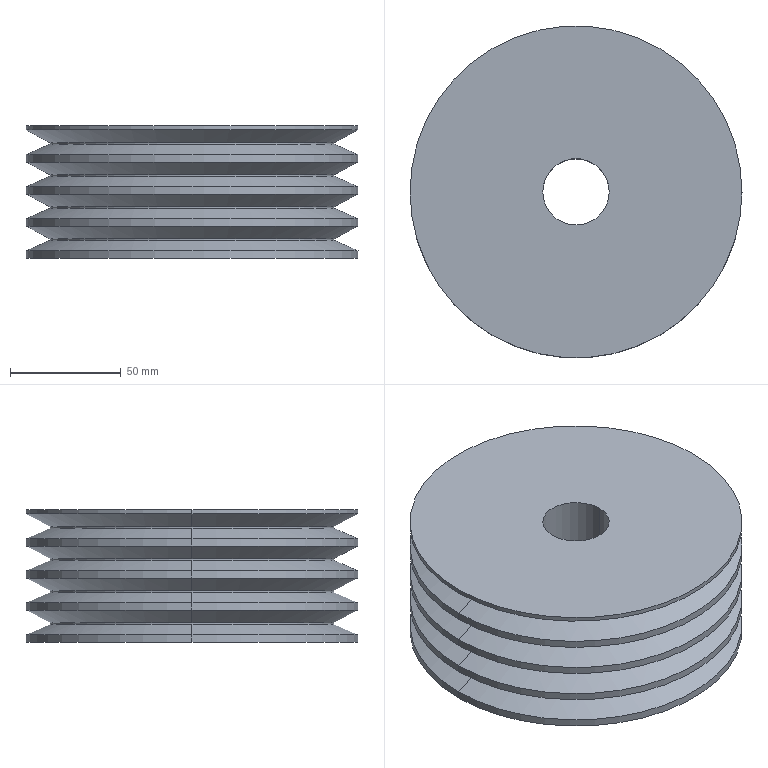Part | SolidWorks | features Extrusion 1, RevCut 1 | 1 solid | 38 faces | box 150 x 150 x 60 mm | volume 903652 mm3 | cylinder 20 | cone 16 | plane 2 | commonest cylinder face diameters 150 x10 128.527 x8 30 x2
STEP:
#1=CARTESIAN_POINT('',(75.,0.,17.907));
#2=VERTEX_POINT('',#1);
#3=CARTESIAN_POINT('',(-75.,0.,17.907));
#4=VERTEX_POINT('',#3);
#5=CARTESIAN_POINT('',(0.,0.,17.907));
#6=DIRECTION('',(0.,0.,1.));
#7=DIRECTION('',(1.,0.,0.));
#8=AXIS2_PLACEMENT_3D('',#5,#6,#7);
#9=CIRCLE('',#8,75.);
#10=EDGE_CURVE('',#2,#4,#9,.T.);
#11=ORIENTED_EDGE('',*,*,#10,.F.);
#12=CARTESIAN_POINT('',(75.,0.,14.583));
#13=VERTEX_POINT('',#12);
#14=CARTESIAN_POINT('',(75.,0.,60.));
#15=DIRECTION('',(0.,0.,-1.));
#16=VECTOR('',#15,1000.);
#17=LINE('',#14,#16);
#18=EDGE_CURVE('',#2,#13,#17,.T.);
#19=ORIENTED_EDGE('',*,*,#18,.T.);
#20=CARTESIAN_POINT('',(-75.,0.,14.583));
#21=VERTEX_POINT('',#20);
#22=CARTESIAN_POINT('',(0.,0.,14.583));
#23=DIRECTION('',(0.,0.,1.));
#24=DIRECTION('',(1.,0.,0.));
#25=AXIS2_PLACEMENT_3D('',#22,#23,#24);
#26=CIRCLE('',#25,75.);
#27=EDGE_CURVE('',#13,#21,#26,.T.);
#28=ORIENTED_EDGE('',*,*,#27,.T.);
#29=CARTESIAN_POINT('',(-75.,0.,60.));
#30=DIRECTION('',(0.,0.,-1.));
#31=VECTOR('',#30,1000.);
#32=LINE('',#29,#31);
#33=EDGE_CURVE('',#4,#21,#32,.T.);
#34=ORIENTED_EDGE('',*,*,#33,.F.);
#35=EDGE_LOOP('',(#11,#19,#28,#34));
#36=FACE_OUTER_BOUND('',#35,.T.);
#37=CARTESIAN_POINT('',(0.,0.,60.));
#38=DIRECTION('',(0.,0.,-1.));
#39=DIRECTION('',(-1.,0.,0.));
#40=AXIS2_PLACEMENT_3D('',#37,#38,#39);
#41=CYLINDRICAL_SURFACE('',#40,75.);
#42=ADVANCED_FACE('',(#36),#41,.T.);
#43=CARTESIAN_POINT('',(64.263,0.,22.613));
#44=VERTEX_POINT('',#43);
#45=CARTESIAN_POINT('',(-64.263,0.,22.613));
#46=VERTEX_POINT('',#45);
#47=CARTESIAN_POINT('',(0.,0.,22.613));
#48=DIRECTION('',(0.,0.,1.));
#49=DIRECTION('',(1.,0.,0.));
#50=AXIS2_PLACEMENT_3D('',#47,#48,#49);
#51=CIRCLE('',#50,64.263);
#52=EDGE_CURVE('',#44,#46,#51,.T.);
#53=ORIENTED_EDGE('',*,*,#52,.T.);
#54=CARTESIAN_POINT('',(-64.263,0.,23.348));
#55=VERTEX_POINT('',#54);
#56=CARTESIAN_POINT('',(-64.263,0.,0.));
#57=DIRECTION('',(0.,0.,1.));
#58=VECTOR('',#57,1000.);
#59=LINE('',#56,#58);
#60=EDGE_CURVE('',#46,#55,#59,.T.);
#61=ORIENTED_EDGE('',*,*,#60,.T.);
#62=CARTESIAN_POINT('',(64.263,0.,23.348));
#63=VERTEX_POINT('',#62);
#64=CARTESIAN_POINT('',(0.,0.,23.348));
#65=DIRECTION('',(0.,0.,1.));
#66=DIRECTION('',(1.,0.,0.));
#67=AXIS2_PLACEMENT_3D('',#64,#65,#66);
#68=CIRCLE('',#67,64.263);
#69=EDGE_CURVE('',#63,#55,#68,.T.);
#70=ORIENTED_EDGE('',*,*,#69,.F.);
#71=CARTESIAN_POINT('',(64.263,0.,0.));
#72=DIRECTION('',(0.,0.,1.));
#73=VECTOR('',#72,1000.);
#74=LINE('',#71,#73);
#75=EDGE_CURVE('',#44,#63,#74,.T.);
#76=ORIENTED_EDGE('',*,*,#75,.F.);
#77=EDGE_LOOP('',(#53,#61,#70,#76));
#78=FACE_OUTER_BOUND('',#77,.T.);
#79=CARTESIAN_POINT('',(0.,0.,0.));
#80=DIRECTION('',(0.,0.,1.));
#81=DIRECTION('',(1.,0.,0.));
#82=AXIS2_PLACEMENT_3D('',#79,#80,#81);
#83=CYLINDRICAL_SURFACE('',#82,64.263);
#84=ADVANCED_FACE('',(#78),#83,.T.);
#85=ORIENTED_EDGE('',*,*,#69,.T.);
#86=CARTESIAN_POINT('',(-75.,0.,29.063));
#87=VERTEX_POINT('',#86);
#88=CARTESIAN_POINT('',(-75.,0.,29.063));
#89=DIRECTION('',(-0.8827,0.,0.4699));
#90=VECTOR('',#89,1000.);
#91=LINE('',#88,#90);
#92=EDGE_CURVE('',#55,#87,#91,.T.);
#93=ORIENTED_EDGE('',*,*,#92,.T.);
#94=CARTESIAN_POINT('',(75.,0.,29.063));
#95=VERTEX_POINT('',#94);
#96=CARTESIAN_POINT('',(0.,0.,29.063));
#97=DIRECTION('',(0.,0.,1.));
#98=DIRECTION('',(1.,0.,0.));
#99=AXIS2_PLACEMENT_3D('',#96,#97,#98);
#100=CIRCLE('',#99,75.);
#101=EDGE_CURVE('',#95,#87,#100,.T.);
#102=ORIENTED_EDGE('',*,*,#101,.F.);
#103=CARTESIAN_POINT('',(75.,0.,29.063));
#104=DIRECTION('',(0.8827,0.,0.4699));
#105=VECTOR('',#104,1000.);
#106=LINE('',#103,#105);
#107=EDGE_CURVE('',#63,#95,#106,.T.);
#108=ORIENTED_EDGE('',*,*,#107,.F.);
#109=EDGE_LOOP('',(#85,#93,#102,#108));
#110=FACE_OUTER_BOUND('',#109,.T.);
#111=CARTESIAN_POINT('',(0.,0.,29.063));
#112=DIRECTION('',(0.,0.,1.));
#113=DIRECTION('',(1.,0.,0.));
#114=AXIS2_PLACEMENT_3D('',#111,#112,#113);
#115=CONICAL_SURFACE('',#114,75.,1.082);
#116=ADVANCED_FACE('',(#110),#115,.T.);
#117=ORIENTED_EDGE('',*,*,#52,.F.);
#118=CARTESIAN_POINT('',(64.263,0.,22.613));
#119=DIRECTION('',(0.9159,0.,-0.4015));
#120=VECTOR('',#119,1000.);
#121=LINE('',#118,#120);
#122=EDGE_CURVE('',#44,#2,#121,.T.);
#123=ORIENTED_EDGE('',*,*,#122,.T.);
#124=ORIENTED_EDGE('',*,*,#10,.T.);
#125=CARTESIAN_POINT('',(-64.263,0.,22.613));
#126=DIRECTION('',(-0.9159,0.,-0.4015));
#127=VECTOR('',#126,1000.);
#128=LINE('',#125,#127);
#129=EDGE_CURVE('',#46,#4,#128,.T.);
#130=ORIENTED_EDGE('',*,*,#129,.F.);
#131=EDGE_LOOP('',(#117,#123,#124,#130));
#132=FACE_OUTER_BOUND('',#131,.T.);
#133=CARTESIAN_POINT('',(0.,0.,22.613));
#134=DIRECTION('',(0.,0.,-1.));
#135=DIRECTION('',(-1.,0.,0.));
#136=AXIS2_PLACEMENT_3D('',#133,#134,#135);
#137=CONICAL_SURFACE('',#136,64.263,1.158);
#138=ADVANCED_FACE('',(#132),#137,.T.);
#139=CARTESIAN_POINT('',(75.,0.,32.387));
#140=VERTEX_POINT('',#139);
#141=CARTESIAN_POINT('',(-75.,0.,32.387));
#142=VERTEX_POINT('',#141);
#143=CARTESIAN_POINT('',(0.,0.,32.387));
#144=DIRECTION('',(0.,0.,1.));
#145=DIRECTION('',(1.,0.,0.));
#146=AXIS2_PLACEMENT_3D('',#143,#144,#145);
#147=CIRCLE('',#146,75.);
#148=EDGE_CURVE('',#140,#142,#147,.T.);
#149=ORIENTED_EDGE('',*,*,#148,.F.);
#150=CARTESIAN_POINT('',(75.,0.,60.));
#151=DIRECTION('',(0.,0.,-1.));
#152=VECTOR('',#151,1000.);
#153=LINE('',#150,#152);
#154=EDGE_CURVE('',#140,#95,#153,.T.);
#155=ORIENTED_EDGE('',*,*,#154,.T.);
#156=ORIENTED_EDGE('',*,*,#101,.T.);
#157=CARTESIAN_POINT('',(-75.,0.,60.));
#158=DIRECTION('',(0.,0.,-1.));
#159=VECTOR('',#158,1000.);
#160=LINE('',#157,#159);
#161=EDGE_CURVE('',#142,#87,#160,.T.);
#162=ORIENTED_EDGE('',*,*,#161,.F.);
#163=EDGE_LOOP('',(#149,#155,#156,#162));
#164=FACE_OUTER_BOUND('',#163,.T.);
#165=CARTESIAN_POINT('',(0.,0.,60.));
#166=DIRECTION('',(0.,0.,-1.));
#167=DIRECTION('',(-1.,0.,0.));
#168=AXIS2_PLACEMENT_3D('',#165,#166,#167);
#169=CYLINDRICAL_SURFACE('',#168,75.);
#170=ADVANCED_FACE('',(#164),#169,.T.);
#171=CARTESIAN_POINT('',(64.263,0.,37.093));
#172=VERTEX_POINT('',#171);
#173=CARTESIAN_POINT('',(-64.263,0.,37.093));
#174=VERTEX_POINT('',#173);
#175=CARTESIAN_POINT('',(0.,0.,37.093));
#176=DIRECTION('',(0.,0.,1.));
#177=DIRECTION('',(1.,0.,0.));
#178=AXIS2_PLACEMENT_3D('',#175,#176,#177);
#179=CIRCLE('',#178,64.263);
#180=EDGE_CURVE('',#172,#174,#179,.T.);
#181=ORIENTED_EDGE('',*,*,#180,.T.);
#182=CARTESIAN_POINT('',(-64.263,0.,37.828));
#183=VERTEX_POINT('',#182);
#184=CARTESIAN_POINT('',(-64.263,0.,0.));
#185=DIRECTION('',(0.,0.,1.));
#186=VECTOR('',#185,1000.);
#187=LINE('',#184,#186);
#188=EDGE_CURVE('',#174,#183,#187,.T.);
#189=ORIENTED_EDGE('',*,*,#188,.T.);
#190=CARTESIAN_POINT('',(64.263,0.,37.828));
#191=VERTEX_POINT('',#190);
#192=CARTESIAN_POINT('',(0.,0.,37.828));
#193=DIRECTION('',(0.,0.,1.));
#194=DIRECTION('',(1.,0.,0.));
#195=AXIS2_PLACEMENT_3D('',#192,#193,#194);
#196=CIRCLE('',#195,64.263);
#197=EDGE_CURVE('',#191,#183,#196,.T.);
#198=ORIENTED_EDGE('',*,*,#197,.F.);
#199=CARTESIAN_POINT('',(64.263,0.,0.));
#200=DIRECTION('',(0.,0.,1.));
#201=VECTOR('',#200,1000.);
#202=LINE('',#199,#201);
#203=EDGE_CURVE('',#172,#191,#202,.T.);
#204=ORIENTED_EDGE('',*,*,#203,.F.);
#205=EDGE_LOOP('',(#181,#189,#198,#204));
#206=FACE_OUTER_BOUND('',#205,.T.);
#207=CARTESIAN_POINT('',(0.,0.,0.));
#208=DIRECTION('',(0.,0.,1.));
#209=DIRECTION('',(1.,0.,0.));
#210=AXIS2_PLACEMENT_3D('',#207,#208,#209);
#211=CYLINDRICAL_SURFACE('',#210,64.263);
#212=ADVANCED_FACE('',(#206),#211,.T.);
#213=ORIENTED_EDGE('',*,*,#197,.T.);
#214=CARTESIAN_POINT('',(-75.,0.,43.543));
#215=VERTEX_POINT('',#214);
#216=CARTESIAN_POINT('',(-75.,0.,43.543));
#217=DIRECTION('',(-0.8827,0.,0.4699));
#218=VECTOR('',#217,1000.);
#219=LINE('',#216,#218);
#220=EDGE_CURVE('',#183,#215,#219,.T.);
#221=ORIENTED_EDGE('',*,*,#220,.T.);
#222=CARTESIAN_POINT('',(75.,0.,43.543));
#223=VERTEX_POINT('',#222);
#224=CARTESIAN_POINT('',(0.,0.,43.543));
#225=DIRECTION('',(0.,0.,1.));
#226=DIRECTION('',(1.,0.,0.));
#227=AXIS2_PLACEMENT_3D('',#224,#225,#226);
#228=CIRCLE('',#227,75.);
#229=EDGE_CURVE('',#223,#215,#228,.T.);
#230=ORIENTED_EDGE('',*,*,#229,.F.);
#231=CARTESIAN_POINT('',(75.,0.,43.543));
#232=DIRECTION('',(0.8827,0.,0.4699));
#233=VECTOR('',#232,1000.);
#234=LINE('',#231,#233);
#235=EDGE_CURVE('',#191,#223,#234,.T.);
#236=ORIENTED_EDGE('',*,*,#235,.F.);
#237=EDGE_LOOP('',(#213,#221,#230,#236));
#238=FACE_OUTER_BOUND('',#237,.T.);
#239=CARTESIAN_POINT('',(0.,0.,43.543));
#240=DIRECTION('',(0.,0.,1.));
#241=DIRECTION('',(1.,0.,0.));
#242=AXIS2_PLACEMENT_3D('',#239,#240,#241);
#243=CONICAL_SURFACE('',#242,75.,1.082);
#244=ADVANCED_FACE('',(#238),#243,.T.);
#245=ORIENTED_EDGE('',*,*,#180,.F.);
#246=CARTESIAN_POINT('',(64.263,0.,37.093));
#247=DIRECTION('',(0.9159,0.,-0.4015));
#248=VECTOR('',#247,1000.);
#249=LINE('',#246,#248);
#250=EDGE_CURVE('',#172,#140,#249,.T.);
#251=ORIENTED_EDGE('',*,*,#250,.T.);
#252=ORIENTED_EDGE('',*,*,#148,.T.);
#253=CARTESIAN_POINT('',(-64.263,0.,37.093));
#254=DIRECTION('',(-0.9159,0.,-0.4015));
#255=VECTOR('',#254,1000.);
#256=LINE('',#253,#255);
#257=EDGE_CURVE('',#174,#142,#256,.T.);
#258=ORIENTED_EDGE('',*,*,#257,.F.);
#259=EDGE_LOOP('',(#245,#251,#252,#258));
#260=FACE_OUTER_BOUND('',#259,.T.);
#261=CARTESIAN_POINT('',(0.,0.,37.093));
#262=DIRECTION('',(0.,0.,-1.));
#263=DIRECTION('',(-1.,0.,0.));
#264=AXIS2_PLACEMENT_3D('',#261,#262,#263);
#265=CONICAL_SURFACE('',#264,64.263,1.158);
#266=ADVANCED_FACE('',(#260),#265,.T.);
#267=CARTESIAN_POINT('',(75.,0.,46.866));
#268=VERTEX_POINT('',#267);
#269=CARTESIAN_POINT('',(-75.,0.,46.866));
#270=VERTEX_POINT('',#269);
#271=CARTESIAN_POINT('',(0.,0.,46.866));
#272=DIRECTION('',(0.,0.,1.));
#273=DIRECTION('',(1.,0.,0.));
#274=AXIS2_PLACEMENT_3D('',#271,#272,#273);
#275=CIRCLE('',#274,75.);
#276=EDGE_CURVE('',#268,#270,#275,.T.);
#277=ORIENTED_EDGE('',*,*,#276,.F.);
#278=CARTESIAN_POINT('',(75.,0.,60.));
#279=DIRECTION('',(0.,0.,-1.));
#280=VECTOR('',#279,1000.);
#281=LINE('',#278,#280);
#282=EDGE_CURVE('',#268,#223,#281,.T.);
#283=ORIENTED_EDGE('',*,*,#282,.T.);
#284=ORIENTED_EDGE('',*,*,#229,.T.);
#285=CARTESIAN_POINT('',(-75.,0.,60.));
#286=DIRECTION('',(0.,0.,-1.));
#287=VECTOR('',#286,1000.);
#288=LINE('',#285,#287);
#289=EDGE_CURVE('',#270,#215,#288,.T.);
#290=ORIENTED_EDGE('',*,*,#289,.F.);
#291=EDGE_LOOP('',(#277,#283,#284,#290));
#292=FACE_OUTER_BOUND('',#291,.T.);
#293=CARTESIAN_POINT('',(0.,0.,60.));
#294=DIRECTION('',(0.,0.,-1.));
#295=DIRECTION('',(-1.,0.,0.));
#296=AXIS2_PLACEMENT_3D('',#293,#294,#295);
#297=CYLINDRICAL_SURFACE('',#296,75.);
#298=ADVANCED_FACE('',(#292),#297,.T.);
#299=CARTESIAN_POINT('',(64.263,0.,8.134));
#300=VERTEX_POINT('',#299);
#301=CARTESIAN_POINT('',(-64.263,0.,8.134));
#302=VERTEX_POINT('',#301);
#303=CARTESIAN_POINT('',(0.,0.,8.134));
#304=DIRECTION('',(0.,0.,1.));
#305=DIRECTION('',(1.,0.,0.));
#306=AXIS2_PLACEMENT_3D('',#303,#304,#305);
#307=CIRCLE('',#306,64.263);
#308=EDGE_CURVE('',#300,#302,#307,.T.);
#309=ORIENTED_EDGE('',*,*,#308,.T.);
#310=CARTESIAN_POINT('',(-64.263,0.,8.868));
#311=VERTEX_POINT('',#310);
#312=CARTESIAN_POINT('',(-64.263,0.,0.));
#313=DIRECTION('',(0.,0.,1.));
#314=VECTOR('',#313,1000.);
#315=LINE('',#312,#314);
#316=EDGE_CURVE('',#302,#311,#315,.T.);
#317=ORIENTED_EDGE('',*,*,#316,.T.);
#318=CARTESIAN_POINT('',(64.263,0.,8.868));
#319=VERTEX_POINT('',#318);
#320=CARTESIAN_POINT('',(0.,0.,8.868));
#321=DIRECTION('',(0.,0.,1.));
#322=DIRECTION('',(1.,0.,0.));
#323=AXIS2_PLACEMENT_3D('',#320,#321,#322);
#324=CIRCLE('',#323,64.263);
#325=EDGE_CURVE('',#319,#311,#324,.T.);
#326=ORIENTED_EDGE('',*,*,#325,.F.);
#327=CARTESIAN_POINT('',(64.263,0.,0.));
#328=DIRECTION('',(0.,0.,1.));
#329=VECTOR('',#328,1000.);
#330=LINE('',#327,#329);
#331=EDGE_CURVE('',#300,#319,#330,.T.);
#332=ORIENTED_EDGE('',*,*,#331,.F.);
#333=EDGE_LOOP('',(#309,#317,#326,#332));
#334=FACE_OUTER_BOUND('',#333,.T.);
#335=CARTESIAN_POINT('',(0.,0.,0.));
#336=DIRECTION('',(0.,0.,1.));
#337=DIRECTION('',(1.,0.,0.));
#338=AXIS2_PLACEMENT_3D('',#335,#336,#337);
#339=CYLINDRICAL_SURFACE('',#338,64.263);
#340=ADVANCED_FACE('',(#334),#339,.T.);
#341=ORIENTED_EDGE('',*,*,#325,.T.);
#342=CARTESIAN_POINT('',(-75.,0.,14.583));
#343=DIRECTION('',(-0.8827,0.,0.4699));
#344=VECTOR('',#343,1000.);
#345=LINE('',#342,#344);
#346=EDGE_CURVE('',#311,#21,#345,.T.);
#347=ORIENTED_EDGE('',*,*,#346,.T.);
#348=ORIENTED_EDGE('',*,*,#27,.F.);
#349=CARTESIAN_POINT('',(75.,0.,14.583));
#350=DIRECTION('',(0.8827,0.,0.4699));
#351=VECTOR('',#350,1000.);
#352=LINE('',#349,#351);
#353=EDGE_CURVE('',#319,#13,#352,.T.);
#354=ORIENTED_EDGE('',*,*,#353,.F.);
#355=EDGE_LOOP('',(#341,#347,#348,#354));
#356=FACE_OUTER_BOUND('',#355,.T.);
#357=CARTESIAN_POINT('',(0.,0.,14.583));
#358=DIRECTION('',(0.,0.,1.));
#359=DIRECTION('',(1.,0.,0.));
#360=AXIS2_PLACEMENT_3D('',#357,#358,#359);
#361=CONICAL_SURFACE('',#360,75.,1.082);
#362=ADVANCED_FACE('',(#356),#361,.T.);
#363=ORIENTED_EDGE('',*,*,#308,.F.);
#364=CARTESIAN_POINT('',(75.,0.,3.427));
#365=VERTEX_POINT('',#364);
#366=CARTESIAN_POINT('',(64.263,0.,8.134));
#367=DIRECTION('',(0.9159,0.,-0.4015));
#368=VECTOR('',#367,1000.);
#369=LINE('',#366,#368);
#370=EDGE_CURVE('',#300,#365,#369,.T.);
#371=ORIENTED_EDGE('',*,*,#370,.T.);
#372=CARTESIAN_POINT('',(-75.,0.,3.427));
#373=VERTEX_POINT('',#372);
#374=CARTESIAN_POINT('',(0.,0.,3.427));
#375=DIRECTION('',(0.,0.,1.));
#376=DIRECTION('',(1.,0.,0.));
#377=AXIS2_PLACEMENT_3D('',#374,#375,#376);
#378=CIRCLE('',#377,75.);
#379=EDGE_CURVE('',#365,#373,#378,.T.);
#380=ORIENTED_EDGE('',*,*,#379,.T.);
#381=CARTESIAN_POINT('',(-64.263,0.,8.134));
#382=DIRECTION('',(-0.9159,0.,-0.4015));
#383=VECTOR('',#382,1000.);
#384=LINE('',#381,#383);
#385=EDGE_CURVE('',#302,#373,#384,.T.);
#386=ORIENTED_EDGE('',*,*,#385,.F.);
#387=EDGE_LOOP('',(#363,#371,#380,#386));
#388=FACE_OUTER_BOUND('',#387,.T.);
#389=CARTESIAN_POINT('',(0.,0.,8.134));
#390=DIRECTION('',(0.,0.,-1.));
#391=DIRECTION('',(-1.,0.,0.));
#392=AXIS2_PLACEMENT_3D('',#389,#390,#391);
#393=CONICAL_SURFACE('',#392,64.263,1.158);
#394=ADVANCED_FACE('',(#388),#393,.T.);
#395=CARTESIAN_POINT('',(64.263,0.,51.573));
#396=VERTEX_POINT('',#395);
#397=CARTESIAN_POINT('',(-64.263,0.,51.573));
#398=VERTEX_POINT('',#397);
#399=CARTESIAN_POINT('',(0.,0.,51.573));
#400=DIRECTION('',(0.,0.,1.));
#401=DIRECTION('',(1.,0.,0.));
#402=AXIS2_PLACEMENT_3D('',#399,#400,#401);
#403=CIRCLE('',#402,64.263);
#404=EDGE_CURVE('',#396,#398,#403,.T.);
#405=ORIENTED_EDGE('',*,*,#404,.T.);
#406=CARTESIAN_POINT('',(-64.263,0.,52.307));
#407=VERTEX_POINT('',#406);
#408=CARTESIAN_POINT('',(-64.263,0.,0.));
#409=DIRECTION('',(0.,0.,1.));
#410=VECTOR('',#409,1000.);
#411=LINE('',#408,#410);
#412=EDGE_CURVE('',#398,#407,#411,.T.);
#413=ORIENTED_EDGE('',*,*,#412,.T.);
#414=CARTESIAN_POINT('',(64.263,0.,52.307));
#415=VERTEX_POINT('',#414);
#416=CARTESIAN_POINT('',(0.,0.,52.307));
#417=DIRECTION('',(0.,0.,1.));
#418=DIRECTION('',(1.,0.,0.));
#419=AXIS2_PLACEMENT_3D('',#416,#417,#418);
#420=CIRCLE('',#419,64.263);
#421=EDGE_CURVE('',#415,#407,#420,.T.);
#422=ORIENTED_EDGE('',*,*,#421,.F.);
#423=CARTESIAN_POINT('',(64.263,0.,0.));
#424=DIRECTION('',(0.,0.,1.));
#425=VECTOR('',#424,1000.);
#426=LINE('',#423,#425);
#427=EDGE_CURVE('',#396,#415,#426,.T.);
#428=ORIENTED_EDGE('',*,*,#427,.F.);
#429=EDGE_LOOP('',(#405,#413,#422,#428));
#430=FACE_OUTER_BOUND('',#429,.T.);
#431=CARTESIAN_POINT('',(0.,0.,0.));
#432=DIRECTION('',(0.,0.,1.));
#433=DIRECTION('',(1.,0.,0.));
#434=AXIS2_PLACEMENT_3D('',#431,#432,#433);
#435=CYLINDRICAL_SURFACE('',#434,64.263);
#436=ADVANCED_FACE('',(#430),#435,.T.);
#437=ORIENTED_EDGE('',*,*,#421,.T.);
#438=CARTESIAN_POINT('',(-75.,0.,58.022));
#439=VERTEX_POINT('',#438);
#440=CARTESIAN_POINT('',(-75.,0.,58.022));
#441=DIRECTION('',(-0.8827,0.,0.4699));
#442=VECTOR('',#441,1000.);
#443=LINE('',#440,#442);
#444=EDGE_CURVE('',#407,#439,#443,.T.);
#445=ORIENTED_EDGE('',*,*,#444,.T.);
#446=CARTESIAN_POINT('',(75.,0.,58.022));
#447=VERTEX_POINT('',#446);
#448=CARTESIAN_POINT('',(0.,0.,58.022));
#449=DIRECTION('',(0.,0.,1.));
#450=DIRECTION('',(1.,0.,0.));
#451=AXIS2_PLACEMENT_3D('',#448,#449,#450);
#452=CIRCLE('',#451,75.);
#453=EDGE_CURVE('',#447,#439,#452,.T.);
#454=ORIENTED_EDGE('',*,*,#453,.F.);
#455=CARTESIAN_POINT('',(75.,0.,58.022));
#456=DIRECTION('',(0.8827,0.,0.4699));
#457=VECTOR('',#456,1000.);
#458=LINE('',#455,#457);
#459=EDGE_CURVE('',#415,#447,#458,.T.);
#460=ORIENTED_EDGE('',*,*,#459,.F.);
#461=EDGE_LOOP('',(#437,#445,#454,#460));
#462=FACE_OUTER_BOUND('',#461,.T.);
#463=CARTESIAN_POINT('',(0.,0.,58.022));
#464=DIRECTION('',(0.,0.,1.));
#465=DIRECTION('',(1.,0.,0.));
#466=AXIS2_PLACEMENT_3D('',#463,#464,#465);
#467=CONICAL_SURFACE('',#466,75.,1.082);
#468=ADVANCED_FACE('',(#462),#467,.T.);
#469=ORIENTED_EDGE('',*,*,#404,.F.);
#470=CARTESIAN_POINT('',(64.263,0.,51.573));
#471=DIRECTION('',(0.9159,0.,-0.4015));
#472=VECTOR('',#471,1000.);
#473=LINE('',#470,#472);
#474=EDGE_CURVE('',#396,#268,#473,.T.);
#475=ORIENTED_EDGE('',*,*,#474,.T.);
#476=ORIENTED_EDGE('',*,*,#276,.T.);
#477=CARTESIAN_POINT('',(-64.263,0.,51.573));
#478=DIRECTION('',(-0.9159,0.,-0.4015));
#479=VECTOR('',#478,1000.);
#480=LINE('',#477,#479);
#481=EDGE_CURVE('',#398,#270,#480,.T.);
#482=ORIENTED_EDGE('',*,*,#481,.F.);
#483=EDGE_LOOP('',(#469,#475,#476,#482));
#484=FACE_OUTER_BOUND('',#483,.T.);
#485=CARTESIAN_POINT('',(0.,0.,51.573));
#486=DIRECTION('',(0.,0.,-1.));
#487=DIRECTION('',(-1.,0.,0.));
#488=AXIS2_PLACEMENT_3D('',#485,#486,#487);
#489=CONICAL_SURFACE('',#488,64.263,1.158);
#490=ADVANCED_FACE('',(#484),#489,.T.);
#491=CARTESIAN_POINT('',(-15.,0.,60.));
#492=VERTEX_POINT('',#491);
#493=CARTESIAN_POINT('',(15.,0.,60.));
#494=VERTEX_POINT('',#493);
#495=CARTESIAN_POINT('',(0.,0.,60.));
#496=DIRECTION('',(0.,0.,1.));
#497=DIRECTION('',(1.,0.,0.));
#498=AXIS2_PLACEMENT_3D('',#495,#496,#497);
#499=CIRCLE('',#498,15.);
#500=EDGE_CURVE('',#492,#494,#499,.T.);
#501=ORIENTED_EDGE('',*,*,#500,.T.);
#502=CARTESIAN_POINT('',(15.,0.,0.));
#503=VERTEX_POINT('',#502);
#504=CARTESIAN_POINT('',(15.,0.,60.));
#505=DIRECTION('',(0.,0.,-1.));
#506=VECTOR('',#505,1000.);
#507=LINE('',#504,#506);
#508=EDGE_CURVE('',#494,#503,#507,.T.);
#509=ORIENTED_EDGE('',*,*,#508,.T.);
#510=CARTESIAN_POINT('',(-15.,0.,0.));
#511=VERTEX_POINT('',#510);
#512=CARTESIAN_POINT('',(0.,0.,0.));
#513=DIRECTION('',(0.,0.,1.));
#514=DIRECTION('',(1.,0.,0.));
#515=AXIS2_PLACEMENT_3D('',#512,#513,#514);
#516=CIRCLE('',#515,15.);
#517=EDGE_CURVE('',#511,#503,#516,.T.);
#518=ORIENTED_EDGE('',*,*,#517,.F.);
#519=CARTESIAN_POINT('',(-15.,0.,60.));
#520=DIRECTION('',(0.,0.,-1.));
#521=VECTOR('',#520,1000.);
#522=LINE('',#519,#521);
#523=EDGE_CURVE('',#492,#511,#522,.T.);
#524=ORIENTED_EDGE('',*,*,#523,.F.);
#525=EDGE_LOOP('',(#501,#509,#518,#524));
#526=FACE_OUTER_BOUND('',#525,.T.);
#527=CARTESIAN_POINT('',(0.,0.,60.));
#528=DIRECTION('',(0.,0.,-1.));
#529=DIRECTION('',(-1.,0.,0.));
#530=AXIS2_PLACEMENT_3D('',#527,#528,#529);
#531=CYLINDRICAL_SURFACE('',#530,15.);
#532=ADVANCED_FACE('',(#526),#531,.F.);
#533=CARTESIAN_POINT('',(75.,0.,60.));
#534=VERTEX_POINT('',#533);
#535=CARTESIAN_POINT('',(-75.,0.,60.));
#536=VERTEX_POINT('',#535);
#537=CARTESIAN_POINT('',(0.,0.,60.));
#538=DIRECTION('',(0.,0.,1.));
#539=DIRECTION('',(1.,0.,0.));
#540=AXIS2_PLACEMENT_3D('',#537,#538,#539);
#541=CIRCLE('',#540,75.);
#542=EDGE_CURVE('',#534,#536,#541,.T.);
#543=ORIENTED_EDGE('',*,*,#542,.F.);
#544=CARTESIAN_POINT('',(75.,0.,60.));
#545=DIRECTION('',(0.,0.,-1.));
#546=VECTOR('',#545,1000.);
#547=LINE('',#544,#546);
#548=EDGE_CURVE('',#534,#447,#547,.T.);
#549=ORIENTED_EDGE('',*,*,#548,.T.);
#550=ORIENTED_EDGE('',*,*,#453,.T.);
#551=CARTESIAN_POINT('',(-75.,0.,60.));
#552=DIRECTION('',(0.,0.,-1.));
#553=VECTOR('',#552,1000.);
#554=LINE('',#551,#553);
#555=EDGE_CURVE('',#536,#439,#554,.T.);
#556=ORIENTED_EDGE('',*,*,#555,.F.);
#557=EDGE_LOOP('',(#543,#549,#550,#556));
#558=FACE_OUTER_BOUND('',#557,.T.);
#559=CARTESIAN_POINT('',(0.,0.,60.));
#560=DIRECTION('',(0.,0.,-1.));
#561=DIRECTION('',(-1.,0.,0.));
#562=AXIS2_PLACEMENT_3D('',#559,#560,#561);
#563=CYLINDRICAL_SURFACE('',#562,75.);
#564=ADVANCED_FACE('',(#558),#563,.T.);
#565=ORIENTED_EDGE('',*,*,#379,.F.);
#566=CARTESIAN_POINT('',(75.,0.,0.));
#567=VERTEX_POINT('',#566);
#568=CARTESIAN_POINT('',(75.,0.,60.));
#569=DIRECTION('',(0.,0.,-1.));
#570=VECTOR('',#569,1000.);
#571=LINE('',#568,#570);
#572=EDGE_CURVE('',#365,#567,#571,.T.);
#573=ORIENTED_EDGE('',*,*,#572,.T.);
#574=CARTESIAN_POINT('',(-75.,0.,0.));
#575=VERTEX_POINT('',#574);
#576=CARTESIAN_POINT('',(0.,0.,0.));
#577=DIRECTION('',(0.,0.,1.));
#578=DIRECTION('',(1.,0.,0.));
#579=AXIS2_PLACEMENT_3D('',#576,#577,#578);
#580=CIRCLE('',#579,75.);
#581=EDGE_CURVE('',#567,#575,#580,.T.);
#582=ORIENTED_EDGE('',*,*,#581,.T.);
#583=CARTESIAN_POINT('',(-75.,0.,60.));
#584=DIRECTION('',(0.,0.,-1.));
#585=VECTOR('',#584,1000.);
#586=LINE('',#583,#585);
#587=EDGE_CURVE('',#373,#575,#586,.T.);
#588=ORIENTED_EDGE('',*,*,#587,.F.);
#589=EDGE_LOOP('',(#565,#573,#582,#588));
#590=FACE_OUTER_BOUND('',#589,.T.);
#591=CARTESIAN_POINT('',(0.,0.,60.));
#592=DIRECTION('',(0.,0.,-1.));
#593=DIRECTION('',(-1.,0.,0.));
#594=AXIS2_PLACEMENT_3D('',#591,#592,#593);
#595=CYLINDRICAL_SURFACE('',#594,75.);
#596=ADVANCED_FACE('',(#590),#595,.T.);
#597=ORIENTED_EDGE('',*,*,#572,.F.);
#598=CARTESIAN_POINT('',(0.,0.,3.427));
#599=DIRECTION('',(0.,0.,1.));
#600=DIRECTION('',(1.,0.,0.));
#601=AXIS2_PLACEMENT_3D('',#598,#599,#600);
#602=CIRCLE('',#601,75.);
#603=EDGE_CURVE('',#373,#365,#602,.T.);
#604=ORIENTED_EDGE('',*,*,#603,.F.);
#605=ORIENTED_EDGE('',*,*,#587,.T.);
#606=CARTESIAN_POINT('',(0.,0.,0.));
#607=DIRECTION('',(0.,0.,1.));
#608=DIRECTION('',(1.,0.,0.));
#609=AXIS2_PLACEMENT_3D('',#606,#607,#608);
#610=CIRCLE('',#609,75.);
#611=EDGE_CURVE('',#575,#567,#610,.T.);
#612=ORIENTED_EDGE('',*,*,#611,.T.);
#613=EDGE_LOOP('',(#597,#604,#605,#612));
#614=FACE_OUTER_BOUND('',#613,.T.);
#615=CARTESIAN_POINT('',(0.,0.,60.));
#616=DIRECTION('',(0.,0.,-1.));
#617=DIRECTION('',(-1.,0.,0.));
#618=AXIS2_PLACEMENT_3D('',#615,#616,#617);
#619=CYLINDRICAL_SURFACE('',#618,75.);
#620=ADVANCED_FACE('',(#614),#619,.T.);
#621=ORIENTED_EDGE('',*,*,#548,.F.);
#622=CARTESIAN_POINT('',(0.,0.,60.));
#623=DIRECTION('',(0.,0.,1.));
#624=DIRECTION('',(1.,0.,0.));
#625=AXIS2_PLACEMENT_3D('',#622,#623,#624);
#626=CIRCLE('',#625,75.);
#627=EDGE_CURVE('',#536,#534,#626,.T.);
#628=ORIENTED_EDGE('',*,*,#627,.F.);
#629=ORIENTED_EDGE('',*,*,#555,.T.);
#630=CARTESIAN_POINT('',(0.,0.,58.022));
#631=DIRECTION('',(0.,0.,1.));
#632=DIRECTION('',(1.,0.,0.));
#633=AXIS2_PLACEMENT_3D('',#630,#631,#632);
#634=CIRCLE('',#633,75.);
#635=EDGE_CURVE('',#439,#447,#634,.T.);
#636=ORIENTED_EDGE('',*,*,#635,.T.);
#637=EDGE_LOOP('',(#621,#628,#629,#636));
#638=FACE_OUTER_BOUND('',#637,.T.);
#639=CARTESIAN_POINT('',(0.,0.,60.));
#640=DIRECTION('',(0.,0.,-1.));
#641=DIRECTION('',(-1.,0.,0.));
#642=AXIS2_PLACEMENT_3D('',#639,#640,#641);
#643=CYLINDRICAL_SURFACE('',#642,75.);
#644=ADVANCED_FACE('',(#638),#643,.T.);
#645=ORIENTED_EDGE('',*,*,#627,.T.);
#646=ORIENTED_EDGE('',*,*,#542,.T.);
#647=EDGE_LOOP('',(#645,#646));
#648=FACE_OUTER_BOUND('',#647,.T.);
#649=ORIENTED_EDGE('',*,*,#500,.F.);
#650=CARTESIAN_POINT('',(0.,0.,60.));
#651=DIRECTION('',(0.,0.,1.));
#652=DIRECTION('',(1.,0.,0.));
#653=AXIS2_PLACEMENT_3D('',#650,#651,#652);
#654=CIRCLE('',#653,15.);
#655=EDGE_CURVE('',#494,#492,#654,.T.);
#656=ORIENTED_EDGE('',*,*,#655,.F.);
#657=EDGE_LOOP('',(#649,#656));
#658=FACE_BOUND('',#657,.T.);
#659=CARTESIAN_POINT('',(0.,0.,60.));
#660=DIRECTION('',(0.,0.,1.));
#661=DIRECTION('',(1.,0.,0.));
#662=AXIS2_PLACEMENT_3D('',#659,#660,#661);
#663=PLANE('',#662);
#664=ADVANCED_FACE('',(#648,#658),#663,.T.);
#665=ORIENTED_EDGE('',*,*,#611,.F.);
#666=ORIENTED_EDGE('',*,*,#581,.F.);
#667=EDGE_LOOP('',(#665,#666));
#668=FACE_OUTER_BOUND('',#667,.T.);
#669=ORIENTED_EDGE('',*,*,#517,.T.);
#670=CARTESIAN_POINT('',(0.,0.,0.));
#671=DIRECTION('',(0.,0.,1.));
#672=DIRECTION('',(1.,0.,0.));
#673=AXIS2_PLACEMENT_3D('',#670,#671,#672);
#674=CIRCLE('',#673,15.);
#675=EDGE_CURVE('',#503,#511,#674,.T.);
#676=ORIENTED_EDGE('',*,*,#675,.T.);
#677=EDGE_LOOP('',(#669,#676));
#678=FACE_BOUND('',#677,.T.);
#679=CARTESIAN_POINT('',(0.,0.,0.));
#680=DIRECTION('',(0.,0.,1.));
#681=DIRECTION('',(1.,0.,0.));
#682=AXIS2_PLACEMENT_3D('',#679,#680,#681);
#683=PLANE('',#682);
#684=ADVANCED_FACE('',(#668,#678),#683,.F.);
#685=ORIENTED_EDGE('',*,*,#508,.F.);
#686=ORIENTED_EDGE('',*,*,#655,.T.);
#687=ORIENTED_EDGE('',*,*,#523,.T.);
#688=ORIENTED_EDGE('',*,*,#675,.F.);
#689=EDGE_LOOP('',(#685,#686,#687,#688));
#690=FACE_OUTER_BOUND('',#689,.T.);
#691=CARTESIAN_POINT('',(0.,0.,60.));
#692=DIRECTION('',(0.,0.,-1.));
#693=DIRECTION('',(-1.,0.,0.));
#694=AXIS2_PLACEMENT_3D('',#691,#692,#693);
#695=CYLINDRICAL_SURFACE('',#694,15.);
#696=ADVANCED_FACE('',(#690),#695,.F.);
#697=ORIENTED_EDGE('',*,*,#474,.F.);
#698=CARTESIAN_POINT('',(0.,0.,51.573));
#699=DIRECTION('',(0.,0.,1.));
#700=DIRECTION('',(1.,0.,0.));
#701=AXIS2_PLACEMENT_3D('',#698,#699,#700);
#702=CIRCLE('',#701,64.263);
#703=EDGE_CURVE('',#398,#396,#702,.T.);
#704=ORIENTED_EDGE('',*,*,#703,.F.);
#705=ORIENTED_EDGE('',*,*,#481,.T.);
#706=CARTESIAN_POINT('',(0.,0.,46.866));
#707=DIRECTION('',(0.,0.,1.));
#708=DIRECTION('',(1.,0.,0.));
#709=AXIS2_PLACEMENT_3D('',#706,#707,#708);
#710=CIRCLE('',#709,75.);
#711=EDGE_CURVE('',#270,#268,#710,.T.);
#712=ORIENTED_EDGE('',*,*,#711,.T.);
#713=EDGE_LOOP('',(#697,#704,#705,#712));
#714=FACE_OUTER_BOUND('',#713,.T.);
#715=CARTESIAN_POINT('',(0.,0.,51.573));
#716=DIRECTION('',(0.,0.,-1.));
#717=DIRECTION('',(-1.,0.,0.));
#718=AXIS2_PLACEMENT_3D('',#715,#716,#717);
#719=CONICAL_SURFACE('',#718,64.263,1.158);
#720=ADVANCED_FACE('',(#714),#719,.T.);
#721=ORIENTED_EDGE('',*,*,#444,.F.);
#722=CARTESIAN_POINT('',(0.,0.,52.307));
#723=DIRECTION('',(0.,0.,1.));
#724=DIRECTION('',(1.,0.,0.));
#725=AXIS2_PLACEMENT_3D('',#722,#723,#724);
#726=CIRCLE('',#725,64.263);
#727=EDGE_CURVE('',#407,#415,#726,.T.);
#728=ORIENTED_EDGE('',*,*,#727,.T.);
#729=ORIENTED_EDGE('',*,*,#459,.T.);
#730=ORIENTED_EDGE('',*,*,#635,.F.);
#731=EDGE_LOOP('',(#721,#728,#729,#730));
#732=FACE_OUTER_BOUND('',#731,.T.);
#733=CARTESIAN_POINT('',(0.,0.,58.022));
#734=DIRECTION('',(0.,0.,1.));
#735=DIRECTION('',(1.,0.,0.));
#736=AXIS2_PLACEMENT_3D('',#733,#734,#735);
#737=CONICAL_SURFACE('',#736,75.,1.082);
#738=ADVANCED_FACE('',(#732),#737,.T.);
#739=ORIENTED_EDGE('',*,*,#412,.F.);
#740=ORIENTED_EDGE('',*,*,#703,.T.);
#741=ORIENTED_EDGE('',*,*,#427,.T.);
#742=ORIENTED_EDGE('',*,*,#727,.F.);
#743=EDGE_LOOP('',(#739,#740,#741,#742));
#744=FACE_OUTER_BOUND('',#743,.T.);
#745=CARTESIAN_POINT('',(0.,0.,0.));
#746=DIRECTION('',(0.,0.,1.));
#747=DIRECTION('',(1.,0.,0.));
#748=AXIS2_PLACEMENT_3D('',#745,#746,#747);
#749=CYLINDRICAL_SURFACE('',#748,64.263);
#750=ADVANCED_FACE('',(#744),#749,.T.);
#751=ORIENTED_EDGE('',*,*,#370,.F.);
#752=CARTESIAN_POINT('',(0.,0.,8.134));
#753=DIRECTION('',(0.,0.,1.));
#754=DIRECTION('',(1.,0.,0.));
#755=AXIS2_PLACEMENT_3D('',#752,#753,#754);
#756=CIRCLE('',#755,64.263);
#757=EDGE_CURVE('',#302,#300,#756,.T.);
#758=ORIENTED_EDGE('',*,*,#757,.F.);
#759=ORIENTED_EDGE('',*,*,#385,.T.);
#760=ORIENTED_EDGE('',*,*,#603,.T.);
#761=EDGE_LOOP('',(#751,#758,#759,#760));
#762=FACE_OUTER_BOUND('',#761,.T.);
#763=CARTESIAN_POINT('',(0.,0.,8.134));
#764=DIRECTION('',(0.,0.,-1.));
#765=DIRECTION('',(-1.,0.,0.));
#766=AXIS2_PLACEMENT_3D('',#763,#764,#765);
#767=CONICAL_SURFACE('',#766,64.263,1.158);
#768=ADVANCED_FACE('',(#762),#767,.T.);
#769=ORIENTED_EDGE('',*,*,#346,.F.);
#770=CARTESIAN_POINT('',(0.,0.,8.868));
#771=DIRECTION('',(0.,0.,1.));
#772=DIRECTION('',(1.,0.,0.));
#773=AXIS2_PLACEMENT_3D('',#770,#771,#772);
#774=CIRCLE('',#773,64.263);
#775=EDGE_CURVE('',#311,#319,#774,.T.);
#776=ORIENTED_EDGE('',*,*,#775,.T.);
#777=ORIENTED_EDGE('',*,*,#353,.T.);
#778=CARTESIAN_POINT('',(0.,0.,14.583));
#779=DIRECTION('',(0.,0.,1.));
#780=DIRECTION('',(1.,0.,0.));
#781=AXIS2_PLACEMENT_3D('',#778,#779,#780);
#782=CIRCLE('',#781,75.);
#783=EDGE_CURVE('',#21,#13,#782,.T.);
#784=ORIENTED_EDGE('',*,*,#783,.F.);
#785=EDGE_LOOP('',(#769,#776,#777,#784));
#786=FACE_OUTER_BOUND('',#785,.T.);
#787=CARTESIAN_POINT('',(0.,0.,14.583));
#788=DIRECTION('',(0.,0.,1.));
#789=DIRECTION('',(1.,0.,0.));
#790=AXIS2_PLACEMENT_3D('',#787,#788,#789);
#791=CONICAL_SURFACE('',#790,75.,1.082);
#792=ADVANCED_FACE('',(#786),#791,.T.);
#793=ORIENTED_EDGE('',*,*,#316,.F.);
#794=ORIENTED_EDGE('',*,*,#757,.T.);
#795=ORIENTED_EDGE('',*,*,#331,.T.);
#796=ORIENTED_EDGE('',*,*,#775,.F.);
#797=EDGE_LOOP('',(#793,#794,#795,#796));
#798=FACE_OUTER_BOUND('',#797,.T.);
#799=CARTESIAN_POINT('',(0.,0.,0.));
#800=DIRECTION('',(0.,0.,1.));
#801=DIRECTION('',(1.,0.,0.));
#802=AXIS2_PLACEMENT_3D('',#799,#800,#801);
#803=CYLINDRICAL_SURFACE('',#802,64.263);
#804=ADVANCED_FACE('',(#798),#803,.T.);
#805=ORIENTED_EDGE('',*,*,#282,.F.);
#806=ORIENTED_EDGE('',*,*,#711,.F.);
#807=ORIENTED_EDGE('',*,*,#289,.T.);
#808=CARTESIAN_POINT('',(0.,0.,43.543));
#809=DIRECTION('',(0.,0.,1.));
#810=DIRECTION('',(1.,0.,0.));
#811=AXIS2_PLACEMENT_3D('',#808,#809,#810);
#812=CIRCLE('',#811,75.);
#813=EDGE_CURVE('',#215,#223,#812,.T.);
#814=ORIENTED_EDGE('',*,*,#813,.T.);
#815=EDGE_LOOP('',(#805,#806,#807,#814));
#816=FACE_OUTER_BOUND('',#815,.T.);
#817=CARTESIAN_POINT('',(0.,0.,60.));
#818=DIRECTION('',(0.,0.,-1.));
#819=DIRECTION('',(-1.,0.,0.));
#820=AXIS2_PLACEMENT_3D('',#817,#818,#819);
#821=CYLINDRICAL_SURFACE('',#820,75.);
#822=ADVANCED_FACE('',(#816),#821,.T.);
#823=ORIENTED_EDGE('',*,*,#250,.F.);
#824=CARTESIAN_POINT('',(0.,0.,37.093));
#825=DIRECTION('',(0.,0.,1.));
#826=DIRECTION('',(1.,0.,0.));
#827=AXIS2_PLACEMENT_3D('',#824,#825,#826);
#828=CIRCLE('',#827,64.263);
#829=EDGE_CURVE('',#174,#172,#828,.T.);
#830=ORIENTED_EDGE('',*,*,#829,.F.);
#831=ORIENTED_EDGE('',*,*,#257,.T.);
#832=CARTESIAN_POINT('',(0.,0.,32.387));
#833=DIRECTION('',(0.,0.,1.));
#834=DIRECTION('',(1.,0.,0.));
#835=AXIS2_PLACEMENT_3D('',#832,#833,#834);
#836=CIRCLE('',#835,75.);
#837=EDGE_CURVE('',#142,#140,#836,.T.);
#838=ORIENTED_EDGE('',*,*,#837,.T.);
#839=EDGE_LOOP('',(#823,#830,#831,#838));
#840=FACE_OUTER_BOUND('',#839,.T.);
#841=CARTESIAN_POINT('',(0.,0.,37.093));
#842=DIRECTION('',(0.,0.,-1.));
#843=DIRECTION('',(-1.,0.,0.));
#844=AXIS2_PLACEMENT_3D('',#841,#842,#843);
#845=CONICAL_SURFACE('',#844,64.263,1.158);
#846=ADVANCED_FACE('',(#840),#845,.T.);
#847=ORIENTED_EDGE('',*,*,#220,.F.);
#848=CARTESIAN_POINT('',(0.,0.,37.828));
#849=DIRECTION('',(0.,0.,1.));
#850=DIRECTION('',(1.,0.,0.));
#851=AXIS2_PLACEMENT_3D('',#848,#849,#850);
#852=CIRCLE('',#851,64.263);
#853=EDGE_CURVE('',#183,#191,#852,.T.);
#854=ORIENTED_EDGE('',*,*,#853,.T.);
#855=ORIENTED_EDGE('',*,*,#235,.T.);
#856=ORIENTED_EDGE('',*,*,#813,.F.);
#857=EDGE_LOOP('',(#847,#854,#855,#856));
#858=FACE_OUTER_BOUND('',#857,.T.);
#859=CARTESIAN_POINT('',(0.,0.,43.543));
#860=DIRECTION('',(0.,0.,1.));
#861=DIRECTION('',(1.,0.,0.));
#862=AXIS2_PLACEMENT_3D('',#859,#860,#861);
#863=CONICAL_SURFACE('',#862,75.,1.082);
#864=ADVANCED_FACE('',(#858),#863,.T.);
#865=ORIENTED_EDGE('',*,*,#188,.F.);
#866=ORIENTED_EDGE('',*,*,#829,.T.);
#867=ORIENTED_EDGE('',*,*,#203,.T.);
#868=ORIENTED_EDGE('',*,*,#853,.F.);
#869=EDGE_LOOP('',(#865,#866,#867,#868));
#870=FACE_OUTER_BOUND('',#869,.T.);
#871=CARTESIAN_POINT('',(0.,0.,0.));
#872=DIRECTION('',(0.,0.,1.));
#873=DIRECTION('',(1.,0.,0.));
#874=AXIS2_PLACEMENT_3D('',#871,#872,#873);
#875=CYLINDRICAL_SURFACE('',#874,64.263);
#876=ADVANCED_FACE('',(#870),#875,.T.);
#877=ORIENTED_EDGE('',*,*,#154,.F.);
#878=ORIENTED_EDGE('',*,*,#837,.F.);
#879=ORIENTED_EDGE('',*,*,#161,.T.);
#880=CARTESIAN_POINT('',(0.,0.,29.063));
#881=DIRECTION('',(0.,0.,1.));
#882=DIRECTION('',(1.,0.,0.));
#883=AXIS2_PLACEMENT_3D('',#880,#881,#882);
#884=CIRCLE('',#883,75.);
#885=EDGE_CURVE('',#87,#95,#884,.T.);
#886=ORIENTED_EDGE('',*,*,#885,.T.);
#887=EDGE_LOOP('',(#877,#878,#879,#886));
#888=FACE_OUTER_BOUND('',#887,.T.);
#889=CARTESIAN_POINT('',(0.,0.,60.));
#890=DIRECTION('',(0.,0.,-1.));
#891=DIRECTION('',(-1.,0.,0.));
#892=AXIS2_PLACEMENT_3D('',#889,#890,#891);
#893=CYLINDRICAL_SURFACE('',#892,75.);
#894=ADVANCED_FACE('',(#888),#893,.T.);
#895=ORIENTED_EDGE('',*,*,#122,.F.);
#896=CARTESIAN_POINT('',(0.,0.,22.613));
#897=DIRECTION('',(0.,0.,1.));
#898=DIRECTION('',(1.,0.,0.));
#899=AXIS2_PLACEMENT_3D('',#896,#897,#898);
#900=CIRCLE('',#899,64.263);
#901=EDGE_CURVE('',#46,#44,#900,.T.);
#902=ORIENTED_EDGE('',*,*,#901,.F.);
#903=ORIENTED_EDGE('',*,*,#129,.T.);
#904=CARTESIAN_POINT('',(0.,0.,17.907));
#905=DIRECTION('',(0.,0.,1.));
#906=DIRECTION('',(1.,0.,0.));
#907=AXIS2_PLACEMENT_3D('',#904,#905,#906);
#908=CIRCLE('',#907,75.);
#909=EDGE_CURVE('',#4,#2,#908,.T.);
#910=ORIENTED_EDGE('',*,*,#909,.T.);
#911=EDGE_LOOP('',(#895,#902,#903,#910));
#912=FACE_OUTER_BOUND('',#911,.T.);
#913=CARTESIAN_POINT('',(0.,0.,22.613));
#914=DIRECTION('',(0.,0.,-1.));
#915=DIRECTION('',(-1.,0.,0.));
#916=AXIS2_PLACEMENT_3D('',#913,#914,#915);
#917=CONICAL_SURFACE('',#916,64.263,1.158);
#918=ADVANCED_FACE('',(#912),#917,.T.);
#919=ORIENTED_EDGE('',*,*,#92,.F.);
#920=CARTESIAN_POINT('',(0.,0.,23.348));
#921=DIRECTION('',(0.,0.,1.));
#922=DIRECTION('',(1.,0.,0.));
#923=AXIS2_PLACEMENT_3D('',#920,#921,#922);
#924=CIRCLE('',#923,64.263);
#925=EDGE_CURVE('',#55,#63,#924,.T.);
#926=ORIENTED_EDGE('',*,*,#925,.T.);
#927=ORIENTED_EDGE('',*,*,#107,.T.);
#928=ORIENTED_EDGE('',*,*,#885,.F.);
#929=EDGE_LOOP('',(#919,#926,#927,#928));
#930=FACE_OUTER_BOUND('',#929,.T.);
#931=CARTESIAN_POINT('',(0.,0.,29.063));
#932=DIRECTION('',(0.,0.,1.));
#933=DIRECTION('',(1.,0.,0.));
#934=AXIS2_PLACEMENT_3D('',#931,#932,#933);
#935=CONICAL_SURFACE('',#934,75.,1.082);
#936=ADVANCED_FACE('',(#930),#935,.T.);
#937=ORIENTED_EDGE('',*,*,#60,.F.);
#938=ORIENTED_EDGE('',*,*,#901,.T.);
#939=ORIENTED_EDGE('',*,*,#75,.T.);
#940=ORIENTED_EDGE('',*,*,#925,.F.);
#941=EDGE_LOOP('',(#937,#938,#939,#940));
#942=FACE_OUTER_BOUND('',#941,.T.);
#943=CARTESIAN_POINT('',(0.,0.,0.));
#944=DIRECTION('',(0.,0.,1.));
#945=DIRECTION('',(1.,0.,0.));
#946=AXIS2_PLACEMENT_3D('',#943,#944,#945);
#947=CYLINDRICAL_SURFACE('',#946,64.263);
#948=ADVANCED_FACE('',(#942),#947,.T.);
#949=ORIENTED_EDGE('',*,*,#18,.F.);
#950=ORIENTED_EDGE('',*,*,#909,.F.);
#951=ORIENTED_EDGE('',*,*,#33,.T.);
#952=ORIENTED_EDGE('',*,*,#783,.T.);
#953=EDGE_LOOP('',(#949,#950,#951,#952));
#954=FACE_OUTER_BOUND('',#953,.T.);
#955=CARTESIAN_POINT('',(0.,0.,60.));
#956=DIRECTION('',(0.,0.,-1.));
#957=DIRECTION('',(-1.,0.,0.));
#958=AXIS2_PLACEMENT_3D('',#955,#956,#957);
#959=CYLINDRICAL_SURFACE('',#958,75.);
#960=ADVANCED_FACE('',(#954),#959,.T.);
#961=CLOSED_SHELL('',(#42,#84,#116,#138,#170,#212,#244,#266,#298,#340,#362,#394,#436,#468,#490,#532,#564,#596,#620,#644,#664,#684,#696,#720,#738,#750,#768,#792,#804,#822,#846,#864,#876,#894,#918,#936,#948,#960));
#962=MANIFOLD_SOLID_BREP('',#961);
#963=CARTESIAN_POINT('',(0.,0.,0.));
#964=DIRECTION('',(0.,0.,1.));
#965=DIRECTION('',(1.,0.,0.));
#966=AXIS2_PLACEMENT_3D('',#963,#964,#965);
#967=(LENGTH_UNIT()NAMED_UNIT(*)SI_UNIT(.MILLI.,.METRE.));
#968=UNCERTAINTY_MEASURE_WITH_UNIT(LENGTH_MEASURE(0.00001),#967,'','');
#969=(NAMED_UNIT(*)PLANE_ANGLE_UNIT()SI_UNIT($,.RADIAN.));
#970=(NAMED_UNIT(*)SI_UNIT($,.STERADIAN.)SOLID_ANGLE_UNIT());
#971=(GEOMETRIC_REPRESENTATION_CONTEXT(3)GLOBAL_UNCERTAINTY_ASSIGNED_CONTEXT((#968))GLOBAL_UNIT_ASSIGNED_CONTEXT((#967,#969,#970))REPRESENTATION_CONTEXT('',''));
#972=ADVANCED_BREP_SHAPE_REPRESENTATION('',(#962,#966),#971);